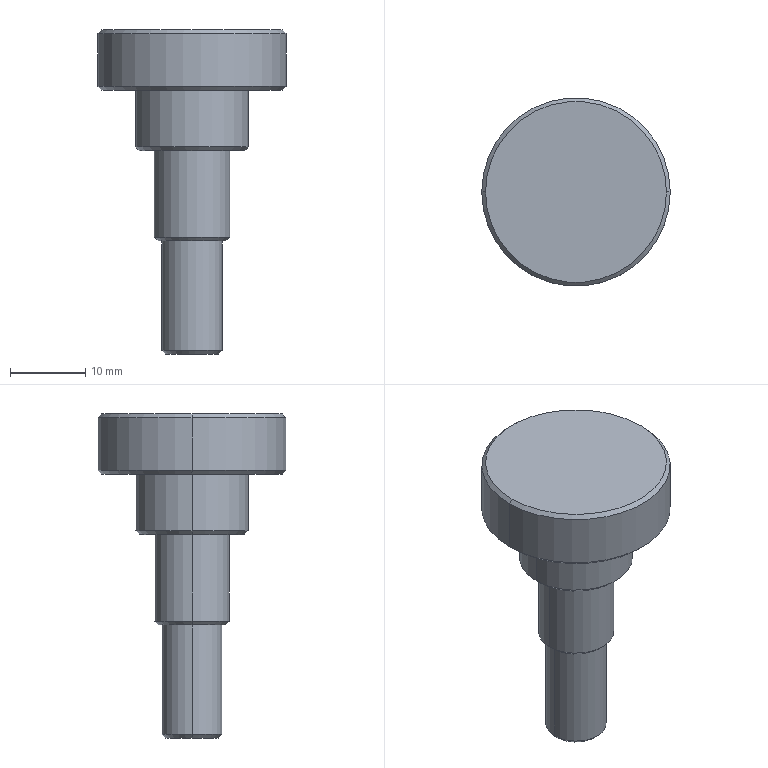Part | SolidWorks | features ICE 3, Chamfer 1, Extrusion 1 | 1 solid | 23 faces | box 25 x 25 x 43 mm | volume 7005 mm3 | cone 10 | cylinder 8 | plane 5 | commonest cylinder face diameters 8 x2 10 x2 15 x2 25 x2
STEP:
#1=CARTESIAN_POINT('',(-3.5,0.,0.));
#2=VERTEX_POINT('',#1);
#3=CARTESIAN_POINT('',(3.5,0.,0.));
#4=VERTEX_POINT('',#3);
#5=CARTESIAN_POINT('',(0.,0.,0.));
#6=DIRECTION('',(0.,0.,-1.));
#7=DIRECTION('',(1.,0.,0.));
#8=AXIS2_PLACEMENT_3D('',#5,#6,#7);
#9=CIRCLE('',#8,3.5);
#10=EDGE_CURVE('',#2,#4,#9,.T.);
#11=ORIENTED_EDGE('',*,*,#10,.F.);
#12=CARTESIAN_POINT('',(-4.,0.,0.5));
#13=VERTEX_POINT('',#12);
#14=CARTESIAN_POINT('',(-4.,0.,0.5));
#15=DIRECTION('',(-0.7071,0.,0.7071));
#16=VECTOR('',#15,1000.);
#17=LINE('',#14,#16);
#18=EDGE_CURVE('',#2,#13,#17,.T.);
#19=ORIENTED_EDGE('',*,*,#18,.T.);
#20=CARTESIAN_POINT('',(4.,0.,0.5));
#21=VERTEX_POINT('',#20);
#22=CARTESIAN_POINT('',(0.,0.,0.5));
#23=DIRECTION('',(0.,0.,1.));
#24=DIRECTION('',(1.,0.,0.));
#25=AXIS2_PLACEMENT_3D('',#22,#23,#24);
#26=CIRCLE('',#25,4.);
#27=EDGE_CURVE('',#21,#13,#26,.T.);
#28=ORIENTED_EDGE('',*,*,#27,.F.);
#29=CARTESIAN_POINT('',(4.,0.,0.5));
#30=DIRECTION('',(0.7071,0.,0.7071));
#31=VECTOR('',#30,1000.);
#32=LINE('',#29,#31);
#33=EDGE_CURVE('',#4,#21,#32,.T.);
#34=ORIENTED_EDGE('',*,*,#33,.F.);
#35=EDGE_LOOP('',(#11,#19,#28,#34));
#36=FACE_OUTER_BOUND('',#35,.T.);
#37=CARTESIAN_POINT('',(0.,0.,0.5));
#38=DIRECTION('',(0.,0.,1.));
#39=DIRECTION('',(1.,0.,0.));
#40=AXIS2_PLACEMENT_3D('',#37,#38,#39);
#41=CONICAL_SURFACE('',#40,4.,0.7854);
#42=ADVANCED_FACE('',(#36),#41,.T.);
#43=CARTESIAN_POINT('',(-4.5,0.,15.));
#44=VERTEX_POINT('',#43);
#45=CARTESIAN_POINT('',(4.5,0.,15.));
#46=VERTEX_POINT('',#45);
#47=CARTESIAN_POINT('',(0.,0.,15.));
#48=DIRECTION('',(0.,0.,-1.));
#49=DIRECTION('',(1.,0.,0.));
#50=AXIS2_PLACEMENT_3D('',#47,#48,#49);
#51=CIRCLE('',#50,4.5);
#52=EDGE_CURVE('',#44,#46,#51,.T.);
#53=ORIENTED_EDGE('',*,*,#52,.F.);
#54=CARTESIAN_POINT('',(-5.,0.,15.5));
#55=VERTEX_POINT('',#54);
#56=CARTESIAN_POINT('',(-5.,0.,15.5));
#57=DIRECTION('',(-0.7071,0.,0.7071));
#58=VECTOR('',#57,1000.);
#59=LINE('',#56,#58);
#60=EDGE_CURVE('',#44,#55,#59,.T.);
#61=ORIENTED_EDGE('',*,*,#60,.T.);
#62=CARTESIAN_POINT('',(5.,0.,15.5));
#63=VERTEX_POINT('',#62);
#64=CARTESIAN_POINT('',(0.,0.,15.5));
#65=DIRECTION('',(0.,0.,1.));
#66=DIRECTION('',(1.,0.,0.));
#67=AXIS2_PLACEMENT_3D('',#64,#65,#66);
#68=CIRCLE('',#67,5.);
#69=EDGE_CURVE('',#63,#55,#68,.T.);
#70=ORIENTED_EDGE('',*,*,#69,.F.);
#71=CARTESIAN_POINT('',(5.,0.,15.5));
#72=DIRECTION('',(0.7071,0.,0.7071));
#73=VECTOR('',#72,1000.);
#74=LINE('',#71,#73);
#75=EDGE_CURVE('',#46,#63,#74,.T.);
#76=ORIENTED_EDGE('',*,*,#75,.F.);
#77=EDGE_LOOP('',(#53,#61,#70,#76));
#78=FACE_OUTER_BOUND('',#77,.T.);
#79=CARTESIAN_POINT('',(0.,0.,15.5));
#80=DIRECTION('',(0.,0.,1.));
#81=DIRECTION('',(1.,0.,0.));
#82=AXIS2_PLACEMENT_3D('',#79,#80,#81);
#83=CONICAL_SURFACE('',#82,5.,0.7854);
#84=ADVANCED_FACE('',(#78),#83,.T.);
#85=CARTESIAN_POINT('',(-7.,0.,27.));
#86=VERTEX_POINT('',#85);
#87=CARTESIAN_POINT('',(7.,0.,27.));
#88=VERTEX_POINT('',#87);
#89=CARTESIAN_POINT('',(0.,0.,27.));
#90=DIRECTION('',(0.,0.,-1.));
#91=DIRECTION('',(1.,0.,0.));
#92=AXIS2_PLACEMENT_3D('',#89,#90,#91);
#93=CIRCLE('',#92,7.);
#94=EDGE_CURVE('',#86,#88,#93,.T.);
#95=ORIENTED_EDGE('',*,*,#94,.F.);
#96=CARTESIAN_POINT('',(-7.5,0.,27.5));
#97=VERTEX_POINT('',#96);
#98=CARTESIAN_POINT('',(-7.5,0.,27.5));
#99=DIRECTION('',(-0.7071,0.,0.7071));
#100=VECTOR('',#99,1000.);
#101=LINE('',#98,#100);
#102=EDGE_CURVE('',#86,#97,#101,.T.);
#103=ORIENTED_EDGE('',*,*,#102,.T.);
#104=CARTESIAN_POINT('',(7.5,0.,27.5));
#105=VERTEX_POINT('',#104);
#106=CARTESIAN_POINT('',(0.,0.,27.5));
#107=DIRECTION('',(0.,0.,1.));
#108=DIRECTION('',(1.,0.,0.));
#109=AXIS2_PLACEMENT_3D('',#106,#107,#108);
#110=CIRCLE('',#109,7.5);
#111=EDGE_CURVE('',#105,#97,#110,.T.);
#112=ORIENTED_EDGE('',*,*,#111,.F.);
#113=CARTESIAN_POINT('',(7.5,0.,27.5));
#114=DIRECTION('',(0.7071,0.,0.7071));
#115=VECTOR('',#114,1000.);
#116=LINE('',#113,#115);
#117=EDGE_CURVE('',#88,#105,#116,.T.);
#118=ORIENTED_EDGE('',*,*,#117,.F.);
#119=EDGE_LOOP('',(#95,#103,#112,#118));
#120=FACE_OUTER_BOUND('',#119,.T.);
#121=CARTESIAN_POINT('',(0.,0.,27.5));
#122=DIRECTION('',(0.,0.,1.));
#123=DIRECTION('',(1.,0.,0.));
#124=AXIS2_PLACEMENT_3D('',#121,#122,#123);
#125=CONICAL_SURFACE('',#124,7.5,0.7854);
#126=ADVANCED_FACE('',(#120),#125,.T.);
#127=CARTESIAN_POINT('',(-12.,0.,35.));
#128=VERTEX_POINT('',#127);
#129=CARTESIAN_POINT('',(12.,0.,35.));
#130=VERTEX_POINT('',#129);
#131=CARTESIAN_POINT('',(0.,0.,35.));
#132=DIRECTION('',(0.,0.,-1.));
#133=DIRECTION('',(1.,0.,0.));
#134=AXIS2_PLACEMENT_3D('',#131,#132,#133);
#135=CIRCLE('',#134,12.);
#136=EDGE_CURVE('',#128,#130,#135,.T.);
#137=ORIENTED_EDGE('',*,*,#136,.F.);
#138=CARTESIAN_POINT('',(-12.5,0.,35.5));
#139=VERTEX_POINT('',#138);
#140=CARTESIAN_POINT('',(-12.5,0.,35.5));
#141=DIRECTION('',(-0.7071,0.,0.7071));
#142=VECTOR('',#141,1000.);
#143=LINE('',#140,#142);
#144=EDGE_CURVE('',#128,#139,#143,.T.);
#145=ORIENTED_EDGE('',*,*,#144,.T.);
#146=CARTESIAN_POINT('',(12.5,0.,35.5));
#147=VERTEX_POINT('',#146);
#148=CARTESIAN_POINT('',(0.,0.,35.5));
#149=DIRECTION('',(0.,0.,1.));
#150=DIRECTION('',(1.,0.,0.));
#151=AXIS2_PLACEMENT_3D('',#148,#149,#150);
#152=CIRCLE('',#151,12.5);
#153=EDGE_CURVE('',#147,#139,#152,.T.);
#154=ORIENTED_EDGE('',*,*,#153,.F.);
#155=CARTESIAN_POINT('',(12.5,0.,35.5));
#156=DIRECTION('',(0.7071,0.,0.7071));
#157=VECTOR('',#156,1000.);
#158=LINE('',#155,#157);
#159=EDGE_CURVE('',#130,#147,#158,.T.);
#160=ORIENTED_EDGE('',*,*,#159,.F.);
#161=EDGE_LOOP('',(#137,#145,#154,#160));
#162=FACE_OUTER_BOUND('',#161,.T.);
#163=CARTESIAN_POINT('',(0.,0.,35.5));
#164=DIRECTION('',(0.,0.,1.));
#165=DIRECTION('',(1.,0.,0.));
#166=AXIS2_PLACEMENT_3D('',#163,#164,#165);
#167=CONICAL_SURFACE('',#166,12.5,0.7854);
#168=ADVANCED_FACE('',(#162),#167,.T.);
#169=CARTESIAN_POINT('',(12.,0.,43.));
#170=VERTEX_POINT('',#169);
#171=CARTESIAN_POINT('',(-12.,0.,43.));
#172=VERTEX_POINT('',#171);
#173=CARTESIAN_POINT('',(0.,0.,43.));
#174=DIRECTION('',(0.,0.,1.));
#175=DIRECTION('',(1.,0.,0.));
#176=AXIS2_PLACEMENT_3D('',#173,#174,#175);
#177=CIRCLE('',#176,12.);
#178=EDGE_CURVE('',#170,#172,#177,.T.);
#179=ORIENTED_EDGE('',*,*,#178,.F.);
#180=CARTESIAN_POINT('',(12.5,0.,42.5));
#181=VERTEX_POINT('',#180);
#182=CARTESIAN_POINT('',(12.,0.,43.));
#183=DIRECTION('',(0.7071,0.,-0.7071));
#184=VECTOR('',#183,1000.);
#185=LINE('',#182,#184);
#186=EDGE_CURVE('',#170,#181,#185,.T.);
#187=ORIENTED_EDGE('',*,*,#186,.T.);
#188=CARTESIAN_POINT('',(-12.5,0.,42.5));
#189=VERTEX_POINT('',#188);
#190=CARTESIAN_POINT('',(0.,0.,42.5));
#191=DIRECTION('',(0.,0.,-1.));
#192=DIRECTION('',(1.,0.,0.));
#193=AXIS2_PLACEMENT_3D('',#190,#191,#192);
#194=CIRCLE('',#193,12.5);
#195=EDGE_CURVE('',#189,#181,#194,.T.);
#196=ORIENTED_EDGE('',*,*,#195,.F.);
#197=CARTESIAN_POINT('',(-12.,0.,43.));
#198=DIRECTION('',(-0.7071,0.,-0.7071));
#199=VECTOR('',#198,1000.);
#200=LINE('',#197,#199);
#201=EDGE_CURVE('',#172,#189,#200,.T.);
#202=ORIENTED_EDGE('',*,*,#201,.F.);
#203=EDGE_LOOP('',(#179,#187,#196,#202));
#204=FACE_OUTER_BOUND('',#203,.T.);
#205=CARTESIAN_POINT('',(0.,0.,43.));
#206=DIRECTION('',(0.,0.,-1.));
#207=DIRECTION('',(-1.,0.,0.));
#208=AXIS2_PLACEMENT_3D('',#205,#206,#207);
#209=CONICAL_SURFACE('',#208,12.,0.7854);
#210=ADVANCED_FACE('',(#204),#209,.T.);
#211=ORIENTED_EDGE('',*,*,#195,.T.);
#212=CARTESIAN_POINT('',(12.5,0.,43.));
#213=DIRECTION('',(0.,0.,-1.));
#214=VECTOR('',#213,1000.);
#215=LINE('',#212,#214);
#216=EDGE_CURVE('',#181,#147,#215,.T.);
#217=ORIENTED_EDGE('',*,*,#216,.T.);
#218=ORIENTED_EDGE('',*,*,#153,.T.);
#219=CARTESIAN_POINT('',(-12.5,0.,43.));
#220=DIRECTION('',(0.,0.,-1.));
#221=VECTOR('',#220,1000.);
#222=LINE('',#219,#221);
#223=EDGE_CURVE('',#189,#139,#222,.T.);
#224=ORIENTED_EDGE('',*,*,#223,.F.);
#225=EDGE_LOOP('',(#211,#217,#218,#224));
#226=FACE_OUTER_BOUND('',#225,.T.);
#227=CARTESIAN_POINT('',(0.,0.,43.));
#228=DIRECTION('',(0.,0.,-1.));
#229=DIRECTION('',(-1.,0.,0.));
#230=AXIS2_PLACEMENT_3D('',#227,#228,#229);
#231=CYLINDRICAL_SURFACE('',#230,12.5);
#232=ADVANCED_FACE('',(#226),#231,.T.);
#233=CARTESIAN_POINT('',(7.5,0.,35.));
#234=VERTEX_POINT('',#233);
#235=CARTESIAN_POINT('',(-7.5,0.,35.));
#236=VERTEX_POINT('',#235);
#237=CARTESIAN_POINT('',(0.,0.,35.));
#238=DIRECTION('',(0.,0.,1.));
#239=DIRECTION('',(1.,0.,0.));
#240=AXIS2_PLACEMENT_3D('',#237,#238,#239);
#241=CIRCLE('',#240,7.5);
#242=EDGE_CURVE('',#234,#236,#241,.T.);
#243=ORIENTED_EDGE('',*,*,#242,.F.);
#244=CARTESIAN_POINT('',(7.5,0.,35.));
#245=DIRECTION('',(0.,0.,-1.));
#246=VECTOR('',#245,1000.);
#247=LINE('',#244,#246);
#248=EDGE_CURVE('',#234,#105,#247,.T.);
#249=ORIENTED_EDGE('',*,*,#248,.T.);
#250=ORIENTED_EDGE('',*,*,#111,.T.);
#251=CARTESIAN_POINT('',(-7.5,0.,35.));
#252=DIRECTION('',(0.,0.,-1.));
#253=VECTOR('',#252,1000.);
#254=LINE('',#251,#253);
#255=EDGE_CURVE('',#236,#97,#254,.T.);
#256=ORIENTED_EDGE('',*,*,#255,.F.);
#257=EDGE_LOOP('',(#243,#249,#250,#256));
#258=FACE_OUTER_BOUND('',#257,.T.);
#259=CARTESIAN_POINT('',(0.,0.,35.));
#260=DIRECTION('',(0.,0.,-1.));
#261=DIRECTION('',(-1.,0.,0.));
#262=AXIS2_PLACEMENT_3D('',#259,#260,#261);
#263=CYLINDRICAL_SURFACE('',#262,7.5);
#264=ADVANCED_FACE('',(#258),#263,.T.);
#265=CARTESIAN_POINT('',(5.,0.,27.));
#266=VERTEX_POINT('',#265);
#267=CARTESIAN_POINT('',(-5.,0.,27.));
#268=VERTEX_POINT('',#267);
#269=CARTESIAN_POINT('',(0.,0.,27.));
#270=DIRECTION('',(0.,0.,1.));
#271=DIRECTION('',(1.,0.,0.));
#272=AXIS2_PLACEMENT_3D('',#269,#270,#271);
#273=CIRCLE('',#272,5.);
#274=EDGE_CURVE('',#266,#268,#273,.T.);
#275=ORIENTED_EDGE('',*,*,#274,.F.);
#276=CARTESIAN_POINT('',(5.,0.,27.));
#277=DIRECTION('',(0.,0.,-1.));
#278=VECTOR('',#277,1000.);
#279=LINE('',#276,#278);
#280=EDGE_CURVE('',#266,#63,#279,.T.);
#281=ORIENTED_EDGE('',*,*,#280,.T.);
#282=ORIENTED_EDGE('',*,*,#69,.T.);
#283=CARTESIAN_POINT('',(-5.,0.,27.));
#284=DIRECTION('',(0.,0.,-1.));
#285=VECTOR('',#284,1000.);
#286=LINE('',#283,#285);
#287=EDGE_CURVE('',#268,#55,#286,.T.);
#288=ORIENTED_EDGE('',*,*,#287,.F.);
#289=EDGE_LOOP('',(#275,#281,#282,#288));
#290=FACE_OUTER_BOUND('',#289,.T.);
#291=CARTESIAN_POINT('',(0.,0.,27.));
#292=DIRECTION('',(0.,0.,-1.));
#293=DIRECTION('',(-1.,0.,0.));
#294=AXIS2_PLACEMENT_3D('',#291,#292,#293);
#295=CYLINDRICAL_SURFACE('',#294,5.);
#296=ADVANCED_FACE('',(#290),#295,.T.);
#297=CARTESIAN_POINT('',(4.,0.,15.));
#298=VERTEX_POINT('',#297);
#299=CARTESIAN_POINT('',(-4.,0.,15.));
#300=VERTEX_POINT('',#299);
#301=CARTESIAN_POINT('',(0.,0.,15.));
#302=DIRECTION('',(0.,0.,1.));
#303=DIRECTION('',(1.,0.,0.));
#304=AXIS2_PLACEMENT_3D('',#301,#302,#303);
#305=CIRCLE('',#304,4.);
#306=EDGE_CURVE('',#298,#300,#305,.T.);
#307=ORIENTED_EDGE('',*,*,#306,.F.);
#308=CARTESIAN_POINT('',(4.,0.,15.));
#309=DIRECTION('',(0.,0.,-1.));
#310=VECTOR('',#309,1000.);
#311=LINE('',#308,#310);
#312=EDGE_CURVE('',#298,#21,#311,.T.);
#313=ORIENTED_EDGE('',*,*,#312,.T.);
#314=ORIENTED_EDGE('',*,*,#27,.T.);
#315=CARTESIAN_POINT('',(-4.,0.,15.));
#316=DIRECTION('',(0.,0.,-1.));
#317=VECTOR('',#316,1000.);
#318=LINE('',#315,#317);
#319=EDGE_CURVE('',#300,#13,#318,.T.);
#320=ORIENTED_EDGE('',*,*,#319,.F.);
#321=EDGE_LOOP('',(#307,#313,#314,#320));
#322=FACE_OUTER_BOUND('',#321,.T.);
#323=CARTESIAN_POINT('',(0.,0.,15.));
#324=DIRECTION('',(0.,0.,-1.));
#325=DIRECTION('',(-1.,0.,0.));
#326=AXIS2_PLACEMENT_3D('',#323,#324,#325);
#327=CYLINDRICAL_SURFACE('',#326,4.);
#328=ADVANCED_FACE('',(#322),#327,.T.);
#329=ORIENTED_EDGE('',*,*,#312,.F.);
#330=CARTESIAN_POINT('',(0.,0.,15.));
#331=DIRECTION('',(0.,0.,1.));
#332=DIRECTION('',(1.,0.,0.));
#333=AXIS2_PLACEMENT_3D('',#330,#331,#332);
#334=CIRCLE('',#333,4.);
#335=EDGE_CURVE('',#300,#298,#334,.T.);
#336=ORIENTED_EDGE('',*,*,#335,.F.);
#337=ORIENTED_EDGE('',*,*,#319,.T.);
#338=CARTESIAN_POINT('',(0.,0.,0.5));
#339=DIRECTION('',(0.,0.,1.));
#340=DIRECTION('',(1.,0.,0.));
#341=AXIS2_PLACEMENT_3D('',#338,#339,#340);
#342=CIRCLE('',#341,4.);
#343=EDGE_CURVE('',#13,#21,#342,.T.);
#344=ORIENTED_EDGE('',*,*,#343,.T.);
#345=EDGE_LOOP('',(#329,#336,#337,#344));
#346=FACE_OUTER_BOUND('',#345,.T.);
#347=CARTESIAN_POINT('',(0.,0.,15.));
#348=DIRECTION('',(0.,0.,-1.));
#349=DIRECTION('',(-1.,0.,0.));
#350=AXIS2_PLACEMENT_3D('',#347,#348,#349);
#351=CYLINDRICAL_SURFACE('',#350,4.);
#352=ADVANCED_FACE('',(#346),#351,.T.);
#353=CARTESIAN_POINT('',(0.,0.,0.));
#354=DIRECTION('',(0.,0.,-1.));
#355=DIRECTION('',(1.,0.,0.));
#356=AXIS2_PLACEMENT_3D('',#353,#354,#355);
#357=CIRCLE('',#356,3.5);
#358=EDGE_CURVE('',#4,#2,#357,.T.);
#359=ORIENTED_EDGE('',*,*,#358,.T.);
#360=ORIENTED_EDGE('',*,*,#10,.T.);
#361=EDGE_LOOP('',(#359,#360));
#362=FACE_OUTER_BOUND('',#361,.T.);
#363=CARTESIAN_POINT('',(0.,0.,0.));
#364=DIRECTION('',(0.,0.,1.));
#365=DIRECTION('',(1.,0.,0.));
#366=AXIS2_PLACEMENT_3D('',#363,#364,#365);
#367=PLANE('',#366);
#368=ADVANCED_FACE('',(#362),#367,.F.);
#369=CARTESIAN_POINT('',(0.,0.,15.));
#370=DIRECTION('',(0.,0.,-1.));
#371=DIRECTION('',(1.,0.,0.));
#372=AXIS2_PLACEMENT_3D('',#369,#370,#371);
#373=CIRCLE('',#372,4.5);
#374=EDGE_CURVE('',#46,#44,#373,.T.);
#375=ORIENTED_EDGE('',*,*,#374,.T.);
#376=ORIENTED_EDGE('',*,*,#52,.T.);
#377=EDGE_LOOP('',(#375,#376));
#378=FACE_OUTER_BOUND('',#377,.T.);
#379=ORIENTED_EDGE('',*,*,#335,.T.);
#380=ORIENTED_EDGE('',*,*,#306,.T.);
#381=EDGE_LOOP('',(#379,#380));
#382=FACE_BOUND('',#381,.T.);
#383=CARTESIAN_POINT('',(0.,0.,15.));
#384=DIRECTION('',(0.,0.,1.));
#385=DIRECTION('',(1.,0.,0.));
#386=AXIS2_PLACEMENT_3D('',#383,#384,#385);
#387=PLANE('',#386);
#388=ADVANCED_FACE('',(#378,#382),#387,.F.);
#389=ORIENTED_EDGE('',*,*,#280,.F.);
#390=CARTESIAN_POINT('',(0.,0.,27.));
#391=DIRECTION('',(0.,0.,1.));
#392=DIRECTION('',(1.,0.,0.));
#393=AXIS2_PLACEMENT_3D('',#390,#391,#392);
#394=CIRCLE('',#393,5.);
#395=EDGE_CURVE('',#268,#266,#394,.T.);
#396=ORIENTED_EDGE('',*,*,#395,.F.);
#397=ORIENTED_EDGE('',*,*,#287,.T.);
#398=CARTESIAN_POINT('',(0.,0.,15.5));
#399=DIRECTION('',(0.,0.,1.));
#400=DIRECTION('',(1.,0.,0.));
#401=AXIS2_PLACEMENT_3D('',#398,#399,#400);
#402=CIRCLE('',#401,5.);
#403=EDGE_CURVE('',#55,#63,#402,.T.);
#404=ORIENTED_EDGE('',*,*,#403,.T.);
#405=EDGE_LOOP('',(#389,#396,#397,#404));
#406=FACE_OUTER_BOUND('',#405,.T.);
#407=CARTESIAN_POINT('',(0.,0.,27.));
#408=DIRECTION('',(0.,0.,-1.));
#409=DIRECTION('',(-1.,0.,0.));
#410=AXIS2_PLACEMENT_3D('',#407,#408,#409);
#411=CYLINDRICAL_SURFACE('',#410,5.);
#412=ADVANCED_FACE('',(#406),#411,.T.);
#413=CARTESIAN_POINT('',(0.,0.,27.));
#414=DIRECTION('',(0.,0.,-1.));
#415=DIRECTION('',(1.,0.,0.));
#416=AXIS2_PLACEMENT_3D('',#413,#414,#415);
#417=CIRCLE('',#416,7.);
#418=EDGE_CURVE('',#88,#86,#417,.T.);
#419=ORIENTED_EDGE('',*,*,#418,.T.);
#420=ORIENTED_EDGE('',*,*,#94,.T.);
#421=EDGE_LOOP('',(#419,#420));
#422=FACE_OUTER_BOUND('',#421,.T.);
#423=ORIENTED_EDGE('',*,*,#395,.T.);
#424=ORIENTED_EDGE('',*,*,#274,.T.);
#425=EDGE_LOOP('',(#423,#424));
#426=FACE_BOUND('',#425,.T.);
#427=CARTESIAN_POINT('',(0.,0.,27.));
#428=DIRECTION('',(0.,0.,1.));
#429=DIRECTION('',(1.,0.,0.));
#430=AXIS2_PLACEMENT_3D('',#427,#428,#429);
#431=PLANE('',#430);
#432=ADVANCED_FACE('',(#422,#426),#431,.F.);
#433=ORIENTED_EDGE('',*,*,#248,.F.);
#434=CARTESIAN_POINT('',(0.,0.,35.));
#435=DIRECTION('',(0.,0.,1.));
#436=DIRECTION('',(1.,0.,0.));
#437=AXIS2_PLACEMENT_3D('',#434,#435,#436);
#438=CIRCLE('',#437,7.5);
#439=EDGE_CURVE('',#236,#234,#438,.T.);
#440=ORIENTED_EDGE('',*,*,#439,.F.);
#441=ORIENTED_EDGE('',*,*,#255,.T.);
#442=CARTESIAN_POINT('',(0.,0.,27.5));
#443=DIRECTION('',(0.,0.,1.));
#444=DIRECTION('',(1.,0.,0.));
#445=AXIS2_PLACEMENT_3D('',#442,#443,#444);
#446=CIRCLE('',#445,7.5);
#447=EDGE_CURVE('',#97,#105,#446,.T.);
#448=ORIENTED_EDGE('',*,*,#447,.T.);
#449=EDGE_LOOP('',(#433,#440,#441,#448));
#450=FACE_OUTER_BOUND('',#449,.T.);
#451=CARTESIAN_POINT('',(0.,0.,35.));
#452=DIRECTION('',(0.,0.,-1.));
#453=DIRECTION('',(-1.,0.,0.));
#454=AXIS2_PLACEMENT_3D('',#451,#452,#453);
#455=CYLINDRICAL_SURFACE('',#454,7.5);
#456=ADVANCED_FACE('',(#450),#455,.T.);
#457=CARTESIAN_POINT('',(0.,0.,35.));
#458=DIRECTION('',(0.,0.,-1.));
#459=DIRECTION('',(1.,0.,0.));
#460=AXIS2_PLACEMENT_3D('',#457,#458,#459);
#461=CIRCLE('',#460,12.);
#462=EDGE_CURVE('',#130,#128,#461,.T.);
#463=ORIENTED_EDGE('',*,*,#462,.T.);
#464=ORIENTED_EDGE('',*,*,#136,.T.);
#465=EDGE_LOOP('',(#463,#464));
#466=FACE_OUTER_BOUND('',#465,.T.);
#467=ORIENTED_EDGE('',*,*,#439,.T.);
#468=ORIENTED_EDGE('',*,*,#242,.T.);
#469=EDGE_LOOP('',(#467,#468));
#470=FACE_BOUND('',#469,.T.);
#471=CARTESIAN_POINT('',(0.,0.,35.));
#472=DIRECTION('',(0.,0.,1.));
#473=DIRECTION('',(1.,0.,0.));
#474=AXIS2_PLACEMENT_3D('',#471,#472,#473);
#475=PLANE('',#474);
#476=ADVANCED_FACE('',(#466,#470),#475,.F.);
#477=ORIENTED_EDGE('',*,*,#216,.F.);
#478=CARTESIAN_POINT('',(0.,0.,42.5));
#479=DIRECTION('',(0.,0.,-1.));
#480=DIRECTION('',(1.,0.,0.));
#481=AXIS2_PLACEMENT_3D('',#478,#479,#480);
#482=CIRCLE('',#481,12.5);
#483=EDGE_CURVE('',#181,#189,#482,.T.);
#484=ORIENTED_EDGE('',*,*,#483,.T.);
#485=ORIENTED_EDGE('',*,*,#223,.T.);
#486=CARTESIAN_POINT('',(0.,0.,35.5));
#487=DIRECTION('',(0.,0.,1.));
#488=DIRECTION('',(1.,0.,0.));
#489=AXIS2_PLACEMENT_3D('',#486,#487,#488);
#490=CIRCLE('',#489,12.5);
#491=EDGE_CURVE('',#139,#147,#490,.T.);
#492=ORIENTED_EDGE('',*,*,#491,.T.);
#493=EDGE_LOOP('',(#477,#484,#485,#492));
#494=FACE_OUTER_BOUND('',#493,.T.);
#495=CARTESIAN_POINT('',(0.,0.,43.));
#496=DIRECTION('',(0.,0.,-1.));
#497=DIRECTION('',(-1.,0.,0.));
#498=AXIS2_PLACEMENT_3D('',#495,#496,#497);
#499=CYLINDRICAL_SURFACE('',#498,12.5);
#500=ADVANCED_FACE('',(#494),#499,.T.);
#501=CARTESIAN_POINT('',(0.,0.,43.));
#502=DIRECTION('',(0.,0.,1.));
#503=DIRECTION('',(1.,0.,0.));
#504=AXIS2_PLACEMENT_3D('',#501,#502,#503);
#505=CIRCLE('',#504,12.);
#506=EDGE_CURVE('',#172,#170,#505,.T.);
#507=ORIENTED_EDGE('',*,*,#506,.T.);
#508=ORIENTED_EDGE('',*,*,#178,.T.);
#509=EDGE_LOOP('',(#507,#508));
#510=FACE_OUTER_BOUND('',#509,.T.);
#511=CARTESIAN_POINT('',(0.,0.,43.));
#512=DIRECTION('',(0.,0.,1.));
#513=DIRECTION('',(1.,0.,0.));
#514=AXIS2_PLACEMENT_3D('',#511,#512,#513);
#515=PLANE('',#514);
#516=ADVANCED_FACE('',(#510),#515,.T.);
#517=ORIENTED_EDGE('',*,*,#186,.F.);
#518=ORIENTED_EDGE('',*,*,#506,.F.);
#519=ORIENTED_EDGE('',*,*,#201,.T.);
#520=ORIENTED_EDGE('',*,*,#483,.F.);
#521=EDGE_LOOP('',(#517,#518,#519,#520));
#522=FACE_OUTER_BOUND('',#521,.T.);
#523=CARTESIAN_POINT('',(0.,0.,43.));
#524=DIRECTION('',(0.,0.,-1.));
#525=DIRECTION('',(-1.,0.,0.));
#526=AXIS2_PLACEMENT_3D('',#523,#524,#525);
#527=CONICAL_SURFACE('',#526,12.,0.7854);
#528=ADVANCED_FACE('',(#522),#527,.T.);
#529=ORIENTED_EDGE('',*,*,#144,.F.);
#530=ORIENTED_EDGE('',*,*,#462,.F.);
#531=ORIENTED_EDGE('',*,*,#159,.T.);
#532=ORIENTED_EDGE('',*,*,#491,.F.);
#533=EDGE_LOOP('',(#529,#530,#531,#532));
#534=FACE_OUTER_BOUND('',#533,.T.);
#535=CARTESIAN_POINT('',(0.,0.,35.5));
#536=DIRECTION('',(0.,0.,1.));
#537=DIRECTION('',(1.,0.,0.));
#538=AXIS2_PLACEMENT_3D('',#535,#536,#537);
#539=CONICAL_SURFACE('',#538,12.5,0.7854);
#540=ADVANCED_FACE('',(#534),#539,.T.);
#541=ORIENTED_EDGE('',*,*,#102,.F.);
#542=ORIENTED_EDGE('',*,*,#418,.F.);
#543=ORIENTED_EDGE('',*,*,#117,.T.);
#544=ORIENTED_EDGE('',*,*,#447,.F.);
#545=EDGE_LOOP('',(#541,#542,#543,#544));
#546=FACE_OUTER_BOUND('',#545,.T.);
#547=CARTESIAN_POINT('',(0.,0.,27.5));
#548=DIRECTION('',(0.,0.,1.));
#549=DIRECTION('',(1.,0.,0.));
#550=AXIS2_PLACEMENT_3D('',#547,#548,#549);
#551=CONICAL_SURFACE('',#550,7.5,0.7854);
#552=ADVANCED_FACE('',(#546),#551,.T.);
#553=ORIENTED_EDGE('',*,*,#60,.F.);
#554=ORIENTED_EDGE('',*,*,#374,.F.);
#555=ORIENTED_EDGE('',*,*,#75,.T.);
#556=ORIENTED_EDGE('',*,*,#403,.F.);
#557=EDGE_LOOP('',(#553,#554,#555,#556));
#558=FACE_OUTER_BOUND('',#557,.T.);
#559=CARTESIAN_POINT('',(0.,0.,15.5));
#560=DIRECTION('',(0.,0.,1.));
#561=DIRECTION('',(1.,0.,0.));
#562=AXIS2_PLACEMENT_3D('',#559,#560,#561);
#563=CONICAL_SURFACE('',#562,5.,0.7854);
#564=ADVANCED_FACE('',(#558),#563,.T.);
#565=ORIENTED_EDGE('',*,*,#18,.F.);
#566=ORIENTED_EDGE('',*,*,#358,.F.);
#567=ORIENTED_EDGE('',*,*,#33,.T.);
#568=ORIENTED_EDGE('',*,*,#343,.F.);
#569=EDGE_LOOP('',(#565,#566,#567,#568));
#570=FACE_OUTER_BOUND('',#569,.T.);
#571=CARTESIAN_POINT('',(0.,0.,0.5));
#572=DIRECTION('',(0.,0.,1.));
#573=DIRECTION('',(1.,0.,0.));
#574=AXIS2_PLACEMENT_3D('',#571,#572,#573);
#575=CONICAL_SURFACE('',#574,4.,0.7854);
#576=ADVANCED_FACE('',(#570),#575,.T.);
#577=CLOSED_SHELL('',(#42,#84,#126,#168,#210,#232,#264,#296,#328,#352,#368,#388,#412,#432,#456,#476,#500,#516,#528,#540,#552,#564,#576));
#578=MANIFOLD_SOLID_BREP('',#577);
#579=CARTESIAN_POINT('',(0.,0.,0.));
#580=DIRECTION('',(0.,0.,1.));
#581=DIRECTION('',(1.,0.,0.));
#582=AXIS2_PLACEMENT_3D('',#579,#580,#581);
#583=(LENGTH_UNIT()NAMED_UNIT(*)SI_UNIT(.MILLI.,.METRE.));
#584=UNCERTAINTY_MEASURE_WITH_UNIT(LENGTH_MEASURE(0.00001),#583,'','');
#585=(NAMED_UNIT(*)PLANE_ANGLE_UNIT()SI_UNIT($,.RADIAN.));
#586=(NAMED_UNIT(*)SI_UNIT($,.STERADIAN.)SOLID_ANGLE_UNIT());
#587=(GEOMETRIC_REPRESENTATION_CONTEXT(3)GLOBAL_UNCERTAINTY_ASSIGNED_CONTEXT((#584))GLOBAL_UNIT_ASSIGNED_CONTEXT((#583,#585,#586))REPRESENTATION_CONTEXT('',''));
#588=ADVANCED_BREP_SHAPE_REPRESENTATION('',(#578,#582),#587);